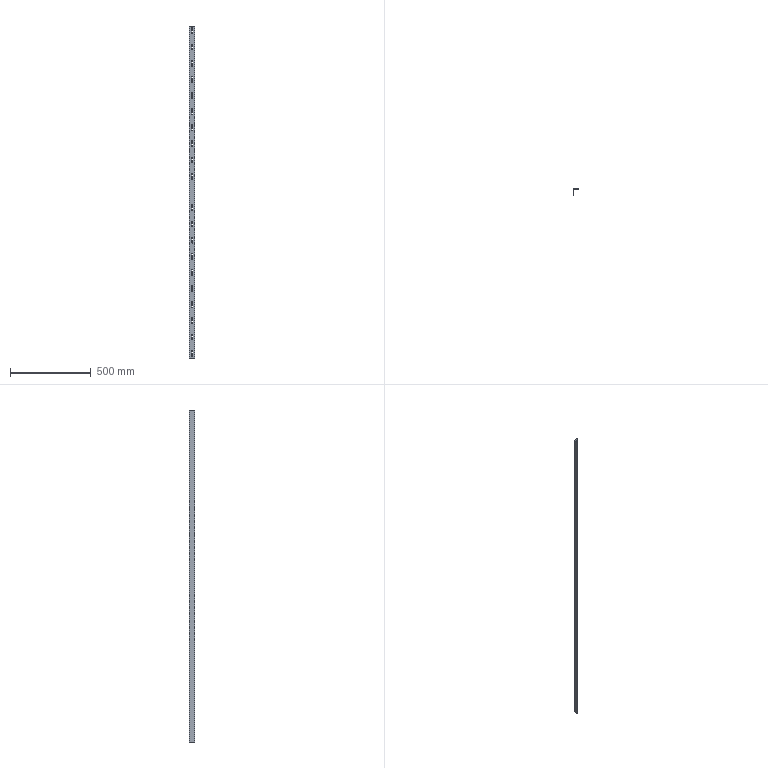Part | SolidWorks | features FlatPattern 1, ICE 1, MirrorPattern 1, SMBaseFlange 1, SheetMetal 1 | 1 solid | 114 faces | box 35 x 35 x 2056 mm | volume 202689 mm3 | cylinder 62 | plane 52 | commonest cylinder face diameters 6 x60 2 x1 5 x1